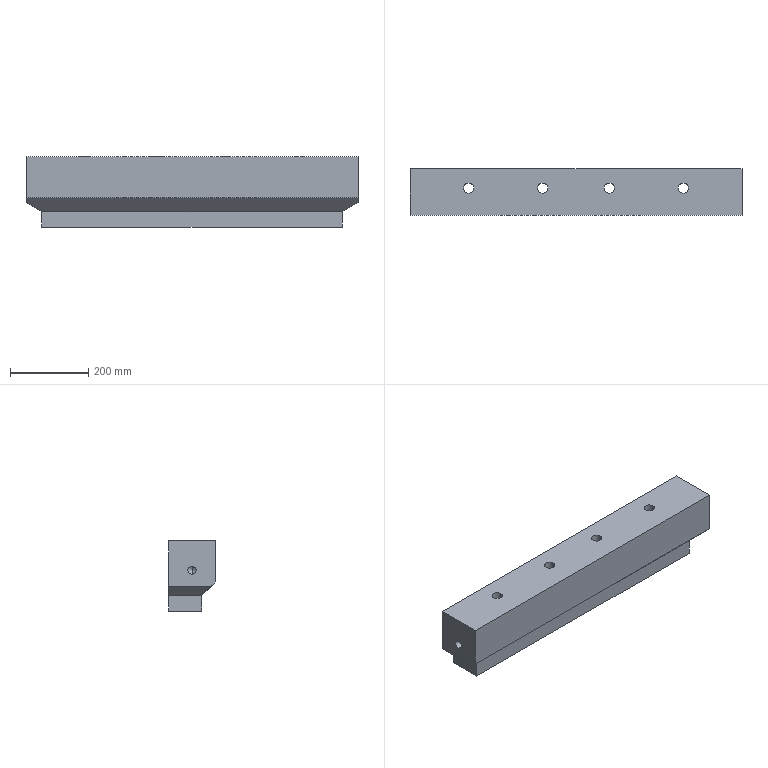Part | SolidWorks | features BaseBody 1 | 1 solid | 50 faces | box 850 x 120 x 180 mm | volume 15854243 mm3 | plane 26 | cylinder 16 | cone 8 | commonest cylinder face diameters 26 x8 17.5 x4 21 x4
STEP:
#1=CARTESIAN_POINT('',(-425.,-295.,-275.));
#2=VERTEX_POINT('',#1);
#3=CARTESIAN_POINT('',(-425.,-295.,-296.));
#4=VERTEX_POINT('',#3);
#5=CARTESIAN_POINT('',(-425.,-295.,-285.5));
#6=DIRECTION('',(1.,0.,0.));
#7=DIRECTION('',(0.,0.,-1.));
#8=AXIS2_PLACEMENT_3D('',#5,#6,#7);
#9=CIRCLE('',#8,10.5);
#10=EDGE_CURVE('',#2,#4,#9,.T.);
#11=ORIENTED_EDGE('',*,*,#10,.F.);
#12=CARTESIAN_POINT('',(-380.,-295.,-275.));
#13=VERTEX_POINT('',#12);
#14=CARTESIAN_POINT('',(-425.,-295.,-275.));
#15=DIRECTION('',(1.,0.,0.));
#16=VECTOR('',#15,1000.);
#17=LINE('',#14,#16);
#18=EDGE_CURVE('',#2,#13,#17,.T.);
#19=ORIENTED_EDGE('',*,*,#18,.T.);
#20=CARTESIAN_POINT('',(-380.,-295.,-296.));
#21=VERTEX_POINT('',#20);
#22=CARTESIAN_POINT('',(-380.,-295.,-285.5));
#23=DIRECTION('',(1.,0.,0.));
#24=DIRECTION('',(0.,0.,-1.));
#25=AXIS2_PLACEMENT_3D('',#22,#23,#24);
#26=CIRCLE('',#25,10.5);
#27=EDGE_CURVE('',#13,#21,#26,.T.);
#28=ORIENTED_EDGE('',*,*,#27,.T.);
#29=CARTESIAN_POINT('',(-425.,-295.,-296.));
#30=DIRECTION('',(1.,0.,0.));
#31=VECTOR('',#30,1000.);
#32=LINE('',#29,#31);
#33=EDGE_CURVE('',#4,#21,#32,.T.);
#34=ORIENTED_EDGE('',*,*,#33,.F.);
#35=EDGE_LOOP('',(#11,#19,#28,#34));
#36=FACE_OUTER_BOUND('',#35,.T.);
#37=CARTESIAN_POINT('',(-425.,-295.,-285.5));
#38=DIRECTION('',(1.,0.,0.));
#39=DIRECTION('',(0.,0.,-1.));
#40=AXIS2_PLACEMENT_3D('',#37,#38,#39);
#41=CYLINDRICAL_SURFACE('',#40,10.5);
#42=ADVANCED_FACE('',(#36),#41,.F.);
#43=CARTESIAN_POINT('',(-373.691,-295.,-285.5));
#44=VERTEX_POINT('',#43);
#45=CARTESIAN_POINT('',(-380.,-295.,-275.));
#46=DIRECTION('',(-0.515,0.,0.8572));
#47=VECTOR('',#46,1000.);
#48=LINE('',#45,#47);
#49=EDGE_CURVE('',#44,#13,#48,.T.);
#50=ORIENTED_EDGE('',*,*,#49,.F.);
#51=CARTESIAN_POINT('',(-380.,-295.,-296.));
#52=DIRECTION('',(-0.515,0.,-0.8572));
#53=VECTOR('',#52,1000.);
#54=LINE('',#51,#53);
#55=EDGE_CURVE('',#44,#21,#54,.T.);
#56=ORIENTED_EDGE('',*,*,#55,.T.);
#57=ORIENTED_EDGE('',*,*,#27,.F.);
#58=EDGE_LOOP('',(#50,#56,#57));
#59=FACE_OUTER_BOUND('',#58,.T.);
#60=CARTESIAN_POINT('',(-380.,-295.,-285.5));
#61=DIRECTION('',(-1.,0.,0.));
#62=DIRECTION('',(0.,0.,1.));
#63=AXIS2_PLACEMENT_3D('',#60,#61,#62);
#64=CONICAL_SURFACE('',#63,10.5,1.03);
#65=ADVANCED_FACE('',(#59),#64,.F.);
#66=CARTESIAN_POINT('',(425.,-295.,-296.));
#67=VERTEX_POINT('',#66);
#68=CARTESIAN_POINT('',(425.,-295.,-275.));
#69=VERTEX_POINT('',#68);
#70=CARTESIAN_POINT('',(425.,-295.,-285.5));
#71=DIRECTION('',(-1.,0.,0.));
#72=DIRECTION('',(0.,0.,1.));
#73=AXIS2_PLACEMENT_3D('',#70,#71,#72);
#74=CIRCLE('',#73,10.5);
#75=EDGE_CURVE('',#67,#69,#74,.T.);
#76=ORIENTED_EDGE('',*,*,#75,.F.);
#77=CARTESIAN_POINT('',(380.,-295.,-296.));
#78=VERTEX_POINT('',#77);
#79=CARTESIAN_POINT('',(425.,-295.,-296.));
#80=DIRECTION('',(-1.,0.,0.));
#81=VECTOR('',#80,1000.);
#82=LINE('',#79,#81);
#83=EDGE_CURVE('',#67,#78,#82,.T.);
#84=ORIENTED_EDGE('',*,*,#83,.T.);
#85=CARTESIAN_POINT('',(380.,-295.,-275.));
#86=VERTEX_POINT('',#85);
#87=CARTESIAN_POINT('',(380.,-295.,-285.5));
#88=DIRECTION('',(-1.,0.,0.));
#89=DIRECTION('',(0.,0.,1.));
#90=AXIS2_PLACEMENT_3D('',#87,#88,#89);
#91=CIRCLE('',#90,10.5);
#92=EDGE_CURVE('',#78,#86,#91,.T.);
#93=ORIENTED_EDGE('',*,*,#92,.T.);
#94=CARTESIAN_POINT('',(425.,-295.,-275.));
#95=DIRECTION('',(-1.,0.,0.));
#96=VECTOR('',#95,1000.);
#97=LINE('',#94,#96);
#98=EDGE_CURVE('',#69,#86,#97,.T.);
#99=ORIENTED_EDGE('',*,*,#98,.F.);
#100=EDGE_LOOP('',(#76,#84,#93,#99));
#101=FACE_OUTER_BOUND('',#100,.T.);
#102=CARTESIAN_POINT('',(425.,-295.,-285.5));
#103=DIRECTION('',(-1.,0.,0.));
#104=DIRECTION('',(0.,0.,1.));
#105=AXIS2_PLACEMENT_3D('',#102,#103,#104);
#106=CYLINDRICAL_SURFACE('',#105,10.5);
#107=ADVANCED_FACE('',(#101),#106,.F.);
#108=CARTESIAN_POINT('',(373.691,-295.,-285.5));
#109=VERTEX_POINT('',#108);
#110=CARTESIAN_POINT('',(380.,-295.,-296.));
#111=DIRECTION('',(0.515,0.,-0.8572));
#112=VECTOR('',#111,1000.);
#113=LINE('',#110,#112);
#114=EDGE_CURVE('',#109,#78,#113,.T.);
#115=ORIENTED_EDGE('',*,*,#114,.F.);
#116=CARTESIAN_POINT('',(380.,-295.,-275.));
#117=DIRECTION('',(0.515,0.,0.8572));
#118=VECTOR('',#117,1000.);
#119=LINE('',#116,#118);
#120=EDGE_CURVE('',#109,#86,#119,.T.);
#121=ORIENTED_EDGE('',*,*,#120,.T.);
#122=ORIENTED_EDGE('',*,*,#92,.F.);
#123=EDGE_LOOP('',(#115,#121,#122));
#124=FACE_OUTER_BOUND('',#123,.T.);
#125=CARTESIAN_POINT('',(380.,-295.,-285.5));
#126=DIRECTION('',(1.,0.,0.));
#127=DIRECTION('',(0.,0.,-1.));
#128=AXIS2_PLACEMENT_3D('',#125,#126,#127);
#129=CONICAL_SURFACE('',#128,10.5,1.03);
#130=ADVANCED_FACE('',(#124),#129,.F.);
#131=CARTESIAN_POINT('',(-353.75,-280.,-390.5));
#132=VERTEX_POINT('',#131);
#133=CARTESIAN_POINT('',(-336.25,-280.,-390.5));
#134=VERTEX_POINT('',#133);
#135=CARTESIAN_POINT('',(-345.,-280.,-390.5));
#136=DIRECTION('',(0.,0.,1.));
#137=DIRECTION('',(1.,0.,0.));
#138=AXIS2_PLACEMENT_3D('',#135,#136,#137);
#139=CIRCLE('',#138,8.75);
#140=EDGE_CURVE('',#132,#134,#139,.T.);
#141=ORIENTED_EDGE('',*,*,#140,.F.);
#142=CARTESIAN_POINT('',(-353.75,-280.,-345.5));
#143=VERTEX_POINT('',#142);
#144=CARTESIAN_POINT('',(-353.75,-280.,-390.5));
#145=DIRECTION('',(0.,0.,1.));
#146=VECTOR('',#145,1000.);
#147=LINE('',#144,#146);
#148=EDGE_CURVE('',#132,#143,#147,.T.);
#149=ORIENTED_EDGE('',*,*,#148,.T.);
#150=CARTESIAN_POINT('',(-336.25,-280.,-345.5));
#151=VERTEX_POINT('',#150);
#152=CARTESIAN_POINT('',(-345.,-280.,-345.5));
#153=DIRECTION('',(0.,0.,1.));
#154=DIRECTION('',(1.,0.,0.));
#155=AXIS2_PLACEMENT_3D('',#152,#153,#154);
#156=CIRCLE('',#155,8.75);
#157=EDGE_CURVE('',#143,#151,#156,.T.);
#158=ORIENTED_EDGE('',*,*,#157,.T.);
#159=CARTESIAN_POINT('',(-336.25,-280.,-390.5));
#160=DIRECTION('',(0.,0.,1.));
#161=VECTOR('',#160,1000.);
#162=LINE('',#159,#161);
#163=EDGE_CURVE('',#134,#151,#162,.T.);
#164=ORIENTED_EDGE('',*,*,#163,.F.);
#165=EDGE_LOOP('',(#141,#149,#158,#164));
#166=FACE_OUTER_BOUND('',#165,.T.);
#167=CARTESIAN_POINT('',(-345.,-280.,-390.5));
#168=DIRECTION('',(0.,0.,1.));
#169=DIRECTION('',(1.,0.,0.));
#170=AXIS2_PLACEMENT_3D('',#167,#168,#169);
#171=CYLINDRICAL_SURFACE('',#170,8.75);
#172=ADVANCED_FACE('',(#166),#171,.F.);
#173=CARTESIAN_POINT('',(-345.,-280.,-340.242));
#174=VERTEX_POINT('',#173);
#175=CARTESIAN_POINT('',(-353.75,-280.,-345.5));
#176=DIRECTION('',(-0.8572,0.,-0.515));
#177=VECTOR('',#176,1000.);
#178=LINE('',#175,#177);
#179=EDGE_CURVE('',#174,#143,#178,.T.);
#180=ORIENTED_EDGE('',*,*,#179,.F.);
#181=CARTESIAN_POINT('',(-336.25,-280.,-345.5));
#182=DIRECTION('',(0.8572,0.,-0.515));
#183=VECTOR('',#182,1000.);
#184=LINE('',#181,#183);
#185=EDGE_CURVE('',#174,#151,#184,.T.);
#186=ORIENTED_EDGE('',*,*,#185,.T.);
#187=ORIENTED_EDGE('',*,*,#157,.F.);
#188=EDGE_LOOP('',(#180,#186,#187));
#189=FACE_OUTER_BOUND('',#188,.T.);
#190=CARTESIAN_POINT('',(-345.,-280.,-345.5));
#191=DIRECTION('',(0.,0.,-1.));
#192=DIRECTION('',(-1.,0.,0.));
#193=AXIS2_PLACEMENT_3D('',#190,#191,#192);
#194=CONICAL_SURFACE('',#193,8.75,1.03);
#195=ADVANCED_FACE('',(#189),#194,.F.);
#196=CARTESIAN_POINT('',(336.25,-280.,-390.5));
#197=VERTEX_POINT('',#196);
#198=CARTESIAN_POINT('',(353.75,-280.,-390.5));
#199=VERTEX_POINT('',#198);
#200=CARTESIAN_POINT('',(345.,-280.,-390.5));
#201=DIRECTION('',(0.,0.,-1.));
#202=DIRECTION('',(-1.,0.,0.));
#203=AXIS2_PLACEMENT_3D('',#200,#201,#202);
#204=CIRCLE('',#203,8.75);
#205=EDGE_CURVE('',#197,#199,#204,.T.);
#206=ORIENTED_EDGE('',*,*,#205,.T.);
#207=CARTESIAN_POINT('',(353.75,-280.,-345.5));
#208=VERTEX_POINT('',#207);
#209=CARTESIAN_POINT('',(353.75,-280.,-390.5));
#210=DIRECTION('',(0.,0.,1.));
#211=VECTOR('',#210,1000.);
#212=LINE('',#209,#211);
#213=EDGE_CURVE('',#199,#208,#212,.T.);
#214=ORIENTED_EDGE('',*,*,#213,.T.);
#215=CARTESIAN_POINT('',(336.25,-280.,-345.5));
#216=VERTEX_POINT('',#215);
#217=CARTESIAN_POINT('',(345.,-280.,-345.5));
#218=DIRECTION('',(0.,0.,-1.));
#219=DIRECTION('',(-1.,0.,0.));
#220=AXIS2_PLACEMENT_3D('',#217,#218,#219);
#221=CIRCLE('',#220,8.75);
#222=EDGE_CURVE('',#216,#208,#221,.T.);
#223=ORIENTED_EDGE('',*,*,#222,.F.);
#224=CARTESIAN_POINT('',(336.25,-280.,-390.5));
#225=DIRECTION('',(0.,0.,1.));
#226=VECTOR('',#225,1000.);
#227=LINE('',#224,#226);
#228=EDGE_CURVE('',#197,#216,#227,.T.);
#229=ORIENTED_EDGE('',*,*,#228,.F.);
#230=EDGE_LOOP('',(#206,#214,#223,#229));
#231=FACE_OUTER_BOUND('',#230,.T.);
#232=CARTESIAN_POINT('',(345.,-280.,-390.5));
#233=DIRECTION('',(0.,0.,1.));
#234=DIRECTION('',(-1.,0.,0.));
#235=AXIS2_PLACEMENT_3D('',#232,#233,#234);
#236=CYLINDRICAL_SURFACE('',#235,8.75);
#237=ADVANCED_FACE('',(#231),#236,.F.);
#238=CARTESIAN_POINT('',(345.,-280.,-340.242));
#239=VERTEX_POINT('',#238);
#240=CARTESIAN_POINT('',(353.75,-280.,-345.5));
#241=DIRECTION('',(0.8572,0.,-0.515));
#242=VECTOR('',#241,1000.);
#243=LINE('',#240,#242);
#244=EDGE_CURVE('',#239,#208,#243,.T.);
#245=ORIENTED_EDGE('',*,*,#244,.F.);
#246=CARTESIAN_POINT('',(336.25,-280.,-345.5));
#247=DIRECTION('',(-0.8572,0.,-0.515));
#248=VECTOR('',#247,1000.);
#249=LINE('',#246,#248);
#250=EDGE_CURVE('',#239,#216,#249,.T.);
#251=ORIENTED_EDGE('',*,*,#250,.T.);
#252=ORIENTED_EDGE('',*,*,#222,.T.);
#253=EDGE_LOOP('',(#245,#251,#252));
#254=FACE_OUTER_BOUND('',#253,.T.);
#255=CARTESIAN_POINT('',(345.,-280.,-345.5));
#256=DIRECTION('',(0.,0.,-1.));
#257=DIRECTION('',(1.,0.,0.));
#258=AXIS2_PLACEMENT_3D('',#255,#256,#257);
#259=CONICAL_SURFACE('',#258,8.75,1.03);
#260=ADVANCED_FACE('',(#254),#259,.F.);
#261=CARTESIAN_POINT('',(-288.,-285.,-390.5));
#262=VERTEX_POINT('',#261);
#263=CARTESIAN_POINT('',(-262.,-285.,-390.5));
#264=VERTEX_POINT('',#263);
#265=CARTESIAN_POINT('',(-275.,-285.,-390.5));
#266=DIRECTION('',(0.,0.,1.));
#267=DIRECTION('',(1.,0.,0.));
#268=AXIS2_PLACEMENT_3D('',#265,#266,#267);
#269=CIRCLE('',#268,13.);
#270=EDGE_CURVE('',#262,#264,#269,.T.);
#271=ORIENTED_EDGE('',*,*,#270,.F.);
#272=CARTESIAN_POINT('',(-288.,-285.,-210.5));
#273=VERTEX_POINT('',#272);
#274=CARTESIAN_POINT('',(-288.,-285.,-395.5));
#275=DIRECTION('',(0.,0.,1.));
#276=VECTOR('',#275,1000.);
#277=LINE('',#274,#276);
#278=EDGE_CURVE('',#262,#273,#277,.T.);
#279=ORIENTED_EDGE('',*,*,#278,.T.);
#280=CARTESIAN_POINT('',(-262.,-285.,-210.5));
#281=VERTEX_POINT('',#280);
#282=CARTESIAN_POINT('',(-275.,-285.,-210.5));
#283=DIRECTION('',(0.,0.,1.));
#284=DIRECTION('',(1.,0.,0.));
#285=AXIS2_PLACEMENT_3D('',#282,#283,#284);
#286=CIRCLE('',#285,13.);
#287=EDGE_CURVE('',#273,#281,#286,.T.);
#288=ORIENTED_EDGE('',*,*,#287,.T.);
#289=CARTESIAN_POINT('',(-262.,-285.,-395.5));
#290=DIRECTION('',(0.,0.,1.));
#291=VECTOR('',#290,1000.);
#292=LINE('',#289,#291);
#293=EDGE_CURVE('',#264,#281,#292,.T.);
#294=ORIENTED_EDGE('',*,*,#293,.F.);
#295=EDGE_LOOP('',(#271,#279,#288,#294));
#296=FACE_OUTER_BOUND('',#295,.T.);
#297=CARTESIAN_POINT('',(-275.,-285.,-395.5));
#298=DIRECTION('',(0.,0.,1.));
#299=DIRECTION('',(1.,0.,0.));
#300=AXIS2_PLACEMENT_3D('',#297,#298,#299);
#301=CYLINDRICAL_SURFACE('',#300,13.);
#302=ADVANCED_FACE('',(#296),#301,.F.);
#303=CARTESIAN_POINT('',(262.,-285.,-390.5));
#304=VERTEX_POINT('',#303);
#305=CARTESIAN_POINT('',(288.,-285.,-390.5));
#306=VERTEX_POINT('',#305);
#307=CARTESIAN_POINT('',(275.,-285.,-390.5));
#308=DIRECTION('',(0.,0.,1.));
#309=DIRECTION('',(1.,0.,0.));
#310=AXIS2_PLACEMENT_3D('',#307,#308,#309);
#311=CIRCLE('',#310,13.);
#312=EDGE_CURVE('',#304,#306,#311,.T.);
#313=ORIENTED_EDGE('',*,*,#312,.F.);
#314=CARTESIAN_POINT('',(262.,-285.,-210.5));
#315=VERTEX_POINT('',#314);
#316=CARTESIAN_POINT('',(262.,-285.,-395.5));
#317=DIRECTION('',(0.,0.,1.));
#318=VECTOR('',#317,1000.);
#319=LINE('',#316,#318);
#320=EDGE_CURVE('',#304,#315,#319,.T.);
#321=ORIENTED_EDGE('',*,*,#320,.T.);
#322=CARTESIAN_POINT('',(288.,-285.,-210.5));
#323=VERTEX_POINT('',#322);
#324=CARTESIAN_POINT('',(275.,-285.,-210.5));
#325=DIRECTION('',(0.,0.,1.));
#326=DIRECTION('',(1.,0.,0.));
#327=AXIS2_PLACEMENT_3D('',#324,#325,#326);
#328=CIRCLE('',#327,13.);
#329=EDGE_CURVE('',#315,#323,#328,.T.);
#330=ORIENTED_EDGE('',*,*,#329,.T.);
#331=CARTESIAN_POINT('',(288.,-285.,-395.5));
#332=DIRECTION('',(0.,0.,1.));
#333=VECTOR('',#332,1000.);
#334=LINE('',#331,#333);
#335=EDGE_CURVE('',#306,#323,#334,.T.);
#336=ORIENTED_EDGE('',*,*,#335,.F.);
#337=EDGE_LOOP('',(#313,#321,#330,#336));
#338=FACE_OUTER_BOUND('',#337,.T.);
#339=CARTESIAN_POINT('',(275.,-285.,-395.5));
#340=DIRECTION('',(0.,0.,1.));
#341=DIRECTION('',(1.,0.,0.));
#342=AXIS2_PLACEMENT_3D('',#339,#340,#341);
#343=CYLINDRICAL_SURFACE('',#342,13.);
#344=ADVANCED_FACE('',(#338),#343,.F.);
#345=CARTESIAN_POINT('',(-98.,-285.,-390.5));
#346=VERTEX_POINT('',#345);
#347=CARTESIAN_POINT('',(-72.,-285.,-390.5));
#348=VERTEX_POINT('',#347);
#349=CARTESIAN_POINT('',(-85.,-285.,-390.5));
#350=DIRECTION('',(0.,0.,1.));
#351=DIRECTION('',(1.,0.,0.));
#352=AXIS2_PLACEMENT_3D('',#349,#350,#351);
#353=CIRCLE('',#352,13.);
#354=EDGE_CURVE('',#346,#348,#353,.T.);
#355=ORIENTED_EDGE('',*,*,#354,.F.);
#356=CARTESIAN_POINT('',(-98.,-285.,-210.5));
#357=VERTEX_POINT('',#356);
#358=CARTESIAN_POINT('',(-98.,-285.,-390.5));
#359=DIRECTION('',(0.,0.,1.));
#360=VECTOR('',#359,1000.);
#361=LINE('',#358,#360);
#362=EDGE_CURVE('',#346,#357,#361,.T.);
#363=ORIENTED_EDGE('',*,*,#362,.T.);
#364=CARTESIAN_POINT('',(-72.,-285.,-210.5));
#365=VERTEX_POINT('',#364);
#366=CARTESIAN_POINT('',(-85.,-285.,-210.5));
#367=DIRECTION('',(0.,0.,1.));
#368=DIRECTION('',(1.,0.,0.));
#369=AXIS2_PLACEMENT_3D('',#366,#367,#368);
#370=CIRCLE('',#369,13.);
#371=EDGE_CURVE('',#357,#365,#370,.T.);
#372=ORIENTED_EDGE('',*,*,#371,.T.);
#373=CARTESIAN_POINT('',(-72.,-285.,-390.5));
#374=DIRECTION('',(0.,0.,1.));
#375=VECTOR('',#374,1000.);
#376=LINE('',#373,#375);
#377=EDGE_CURVE('',#348,#365,#376,.T.);
#378=ORIENTED_EDGE('',*,*,#377,.F.);
#379=EDGE_LOOP('',(#355,#363,#372,#378));
#380=FACE_OUTER_BOUND('',#379,.T.);
#381=CARTESIAN_POINT('',(-85.,-285.,-390.5));
#382=DIRECTION('',(0.,0.,1.));
#383=DIRECTION('',(1.,0.,0.));
#384=AXIS2_PLACEMENT_3D('',#381,#382,#383);
#385=CYLINDRICAL_SURFACE('',#384,13.);
#386=ADVANCED_FACE('',(#380),#385,.F.);
#387=CARTESIAN_POINT('',(72.,-285.,-390.5));
#388=VERTEX_POINT('',#387);
#389=CARTESIAN_POINT('',(98.,-285.,-390.5));
#390=VERTEX_POINT('',#389);
#391=CARTESIAN_POINT('',(85.,-285.,-390.5));
#392=DIRECTION('',(0.,0.,1.));
#393=DIRECTION('',(1.,0.,0.));
#394=AXIS2_PLACEMENT_3D('',#391,#392,#393);
#395=CIRCLE('',#394,13.);
#396=EDGE_CURVE('',#388,#390,#395,.T.);
#397=ORIENTED_EDGE('',*,*,#396,.F.);
#398=CARTESIAN_POINT('',(72.,-285.,-210.5));
#399=VERTEX_POINT('',#398);
#400=CARTESIAN_POINT('',(72.,-285.,-390.5));
#401=DIRECTION('',(0.,0.,1.));
#402=VECTOR('',#401,1000.);
#403=LINE('',#400,#402);
#404=EDGE_CURVE('',#388,#399,#403,.T.);
#405=ORIENTED_EDGE('',*,*,#404,.T.);
#406=CARTESIAN_POINT('',(98.,-285.,-210.5));
#407=VERTEX_POINT('',#406);
#408=CARTESIAN_POINT('',(85.,-285.,-210.5));
#409=DIRECTION('',(0.,0.,1.));
#410=DIRECTION('',(1.,0.,0.));
#411=AXIS2_PLACEMENT_3D('',#408,#409,#410);
#412=CIRCLE('',#411,13.);
#413=EDGE_CURVE('',#399,#407,#412,.T.);
#414=ORIENTED_EDGE('',*,*,#413,.T.);
#415=CARTESIAN_POINT('',(98.,-285.,-390.5));
#416=DIRECTION('',(0.,0.,1.));
#417=VECTOR('',#416,1000.);
#418=LINE('',#415,#417);
#419=EDGE_CURVE('',#390,#407,#418,.T.);
#420=ORIENTED_EDGE('',*,*,#419,.F.);
#421=EDGE_LOOP('',(#397,#405,#414,#420));
#422=FACE_OUTER_BOUND('',#421,.T.);
#423=CARTESIAN_POINT('',(85.,-285.,-390.5));
#424=DIRECTION('',(0.,0.,1.));
#425=DIRECTION('',(1.,0.,0.));
#426=AXIS2_PLACEMENT_3D('',#423,#424,#425);
#427=CYLINDRICAL_SURFACE('',#426,13.);
#428=ADVANCED_FACE('',(#422),#427,.F.);
#429=CARTESIAN_POINT('',(-425.,-295.,-285.5));
#430=DIRECTION('',(1.,0.,0.));
#431=DIRECTION('',(0.,0.,-1.));
#432=AXIS2_PLACEMENT_3D('',#429,#430,#431);
#433=CIRCLE('',#432,10.5);
#434=EDGE_CURVE('',#4,#2,#433,.T.);
#435=ORIENTED_EDGE('',*,*,#434,.T.);
#436=ORIENTED_EDGE('',*,*,#10,.T.);
#437=EDGE_LOOP('',(#435,#436));
#438=FACE_BOUND('',#437,.T.);
#439=CARTESIAN_POINT('',(-425.,-235.,-327.406));
#440=VERTEX_POINT('',#439);
#441=CARTESIAN_POINT('',(-425.,-235.,-210.5));
#442=VERTEX_POINT('',#441);
#443=CARTESIAN_POINT('',(-425.,-235.,-390.5));
#444=DIRECTION('',(0.,0.,1.));
#445=VECTOR('',#444,1000.);
#446=LINE('',#443,#445);
#447=EDGE_CURVE('',#440,#442,#446,.T.);
#448=ORIENTED_EDGE('',*,*,#447,.F.);
#449=CARTESIAN_POINT('',(-425.,-343.094,-327.406));
#450=VERTEX_POINT('',#449);
#451=CARTESIAN_POINT('',(-425.,277.5,-327.406));
#452=DIRECTION('',(0.,-1.,0.));
#453=VECTOR('',#452,1000.);
#454=LINE('',#451,#453);
#455=EDGE_CURVE('',#440,#450,#454,.T.);
#456=ORIENTED_EDGE('',*,*,#455,.T.);
#457=CARTESIAN_POINT('',(-425.,-355.,-315.5));
#458=VERTEX_POINT('',#457);
#459=CARTESIAN_POINT('',(-425.,-320.,-350.5));
#460=DIRECTION('',(0.,-0.7071,0.7071));
#461=VECTOR('',#460,1000.);
#462=LINE('',#459,#461);
#463=EDGE_CURVE('',#450,#458,#462,.T.);
#464=ORIENTED_EDGE('',*,*,#463,.T.);
#465=CARTESIAN_POINT('',(-425.,-355.,-210.5));
#466=VERTEX_POINT('',#465);
#467=CARTESIAN_POINT('',(-425.,-355.,-390.5));
#468=DIRECTION('',(0.,0.,1.));
#469=VECTOR('',#468,1000.);
#470=LINE('',#467,#469);
#471=EDGE_CURVE('',#458,#466,#470,.T.);
#472=ORIENTED_EDGE('',*,*,#471,.T.);
#473=CARTESIAN_POINT('',(-425.,-235.,-210.5));
#474=DIRECTION('',(0.,-1.,0.));
#475=VECTOR('',#474,1000.);
#476=LINE('',#473,#475);
#477=EDGE_CURVE('',#442,#466,#476,.T.);
#478=ORIENTED_EDGE('',*,*,#477,.F.);
#479=EDGE_LOOP('',(#448,#456,#464,#472,#478));
#480=FACE_OUTER_BOUND('',#479,.T.);
#481=CARTESIAN_POINT('',(-425.,-235.,-390.5));
#482=DIRECTION('',(-1.,0.,0.));
#483=DIRECTION('',(0.,-1.,0.));
#484=AXIS2_PLACEMENT_3D('',#481,#482,#483);
#485=PLANE('',#484);
#486=ADVANCED_FACE('',(#438,#480),#485,.T.);
#487=CARTESIAN_POINT('',(375.662,-297.777,-390.5));
#488=VERTEX_POINT('',#487);
#489=CARTESIAN_POINT('',(375.662,-289.777,-390.5));
#490=VERTEX_POINT('',#489);
#491=CARTESIAN_POINT('',(375.662,-297.777,-390.5));
#492=DIRECTION('',(0.,1.,0.));
#493=VECTOR('',#492,1000.);
#494=LINE('',#491,#493);
#495=EDGE_CURVE('',#488,#490,#494,.T.);
#496=ORIENTED_EDGE('',*,*,#495,.F.);
#497=CARTESIAN_POINT('',(365.662,-297.777,-390.5));
#498=VERTEX_POINT('',#497);
#499=CARTESIAN_POINT('',(375.662,-297.777,-390.5));
#500=DIRECTION('',(-1.,0.,0.));
#501=VECTOR('',#500,1000.);
#502=LINE('',#499,#501);
#503=EDGE_CURVE('',#488,#498,#502,.T.);
#504=ORIENTED_EDGE('',*,*,#503,.T.);
#505=CARTESIAN_POINT('',(365.662,-307.777,-390.5));
#506=VERTEX_POINT('',#505);
#507=CARTESIAN_POINT('',(365.662,-307.777,-390.5));
#508=DIRECTION('',(0.,1.,0.));
#509=VECTOR('',#508,1000.);
#510=LINE('',#507,#509);
#511=EDGE_CURVE('',#506,#498,#510,.T.);
#512=ORIENTED_EDGE('',*,*,#511,.F.);
#513=CARTESIAN_POINT('',(357.662,-307.777,-390.5));
#514=VERTEX_POINT('',#513);
#515=CARTESIAN_POINT('',(365.662,-307.777,-390.5));
#516=DIRECTION('',(-1.,0.,0.));
#517=VECTOR('',#516,1000.);
#518=LINE('',#515,#517);
#519=EDGE_CURVE('',#506,#514,#518,.T.);
#520=ORIENTED_EDGE('',*,*,#519,.T.);
#521=CARTESIAN_POINT('',(357.662,-309.777,-390.5));
#522=VERTEX_POINT('',#521);
#523=CARTESIAN_POINT('',(357.662,-307.777,-390.5));
#524=DIRECTION('',(0.,-1.,0.));
#525=VECTOR('',#524,1000.);
#526=LINE('',#523,#525);
#527=EDGE_CURVE('',#514,#522,#526,.T.);
#528=ORIENTED_EDGE('',*,*,#527,.T.);
#529=CARTESIAN_POINT('',(377.662,-309.777,-390.5));
#530=VERTEX_POINT('',#529);
#531=CARTESIAN_POINT('',(377.662,-309.777,-390.5));
#532=DIRECTION('',(-1.,0.,0.));
#533=VECTOR('',#532,1000.);
#534=LINE('',#531,#533);
#535=EDGE_CURVE('',#530,#522,#534,.T.);
#536=ORIENTED_EDGE('',*,*,#535,.F.);
#537=CARTESIAN_POINT('',(377.662,-289.777,-390.5));
#538=VERTEX_POINT('',#537);
#539=CARTESIAN_POINT('',(377.662,-309.777,-390.5));
#540=DIRECTION('',(0.,1.,0.));
#541=VECTOR('',#540,1000.);
#542=LINE('',#539,#541);
#543=EDGE_CURVE('',#530,#538,#542,.T.);
#544=ORIENTED_EDGE('',*,*,#543,.T.);
#545=CARTESIAN_POINT('',(377.662,-289.777,-390.5));
#546=DIRECTION('',(-1.,0.,0.));
#547=VECTOR('',#546,1000.);
#548=LINE('',#545,#547);
#549=EDGE_CURVE('',#538,#490,#548,.T.);
#550=ORIENTED_EDGE('',*,*,#549,.T.);
#551=EDGE_LOOP('',(#496,#504,#512,#520,#528,#536,#544,#550));
#552=FACE_BOUND('',#551,.T.);
#553=CARTESIAN_POINT('',(-345.,-280.,-390.5));
#554=DIRECTION('',(0.,0.,1.));
#555=DIRECTION('',(1.,0.,0.));
#556=AXIS2_PLACEMENT_3D('',#553,#554,#555);
#557=CIRCLE('',#556,8.75);
#558=EDGE_CURVE('',#134,#132,#557,.T.);
#559=ORIENTED_EDGE('',*,*,#558,.T.);
#560=ORIENTED_EDGE('',*,*,#140,.T.);
#561=EDGE_LOOP('',(#559,#560));
#562=FACE_BOUND('',#561,.T.);
#563=CARTESIAN_POINT('',(-385.,-235.,-390.5));
#564=VERTEX_POINT('',#563);
#565=CARTESIAN_POINT('',(-385.,-320.,-390.5));
#566=VERTEX_POINT('',#565);
#567=CARTESIAN_POINT('',(-385.,-277.5,-390.5));
#568=DIRECTION('',(0.,-1.,0.));
#569=VECTOR('',#568,1000.);
#570=LINE('',#567,#569);
#571=EDGE_CURVE('',#564,#566,#570,.T.);
#572=ORIENTED_EDGE('',*,*,#571,.F.);
#573=CARTESIAN_POINT('',(385.,-235.,-390.5));
#574=VERTEX_POINT('',#573);
#575=CARTESIAN_POINT('',(425.,-235.,-390.5));
#576=DIRECTION('',(-1.,0.,0.));
#577=VECTOR('',#576,1000.);
#578=LINE('',#575,#577);
#579=EDGE_CURVE('',#574,#564,#578,.T.);
#580=ORIENTED_EDGE('',*,*,#579,.F.);
#581=CARTESIAN_POINT('',(385.,-320.,-390.5));
#582=VERTEX_POINT('',#581);
#583=CARTESIAN_POINT('',(385.,-355.,-390.5));
#584=DIRECTION('',(0.,-1.,0.));
#585=VECTOR('',#584,1000.);
#586=LINE('',#583,#585);
#587=EDGE_CURVE('',#574,#582,#586,.T.);
#588=ORIENTED_EDGE('',*,*,#587,.T.);
#589=CARTESIAN_POINT('',(510.,-320.,-390.5));
#590=DIRECTION('',(-1.,0.,0.));
#591=VECTOR('',#590,1000.);
#592=LINE('',#589,#591);
#593=EDGE_CURVE('',#582,#566,#592,.T.);
#594=ORIENTED_EDGE('',*,*,#593,.T.);
#595=EDGE_LOOP('',(#572,#580,#588,#594));
#596=FACE_OUTER_BOUND('',#595,.T.);
#597=CARTESIAN_POINT('',(-85.,-285.,-390.5));
#598=DIRECTION('',(0.,0.,1.));
#599=DIRECTION('',(1.,0.,0.));
#600=AXIS2_PLACEMENT_3D('',#597,#598,#599);
#601=CIRCLE('',#600,13.);
#602=EDGE_CURVE('',#348,#346,#601,.T.);
#603=ORIENTED_EDGE('',*,*,#602,.T.);
#604=ORIENTED_EDGE('',*,*,#354,.T.);
#605=EDGE_LOOP('',(#603,#604));
#606=FACE_BOUND('',#605,.T.);
#607=CARTESIAN_POINT('',(85.,-285.,-390.5));
#608=DIRECTION('',(0.,0.,1.));
#609=DIRECTION('',(1.,0.,0.));
#610=AXIS2_PLACEMENT_3D('',#607,#608,#609);
#611=CIRCLE('',#610,13.);
#612=EDGE_CURVE('',#390,#388,#611,.T.);
#613=ORIENTED_EDGE('',*,*,#612,.T.);
#614=ORIENTED_EDGE('',*,*,#396,.T.);
#615=EDGE_LOOP('',(#613,#614));
#616=FACE_BOUND('',#615,.T.);
#617=CARTESIAN_POINT('',(275.,-285.,-390.5));
#618=DIRECTION('',(0.,0.,1.));
#619=DIRECTION('',(1.,0.,0.));
#620=AXIS2_PLACEMENT_3D('',#617,#618,#619);
#621=CIRCLE('',#620,13.);
#622=EDGE_CURVE('',#306,#304,#621,.T.);
#623=ORIENTED_EDGE('',*,*,#622,.T.);
#624=ORIENTED_EDGE('',*,*,#312,.T.);
#625=EDGE_LOOP('',(#623,#624));
#626=FACE_BOUND('',#625,.T.);
#627=CARTESIAN_POINT('',(-275.,-285.,-390.5));
#628=DIRECTION('',(0.,0.,1.));
#629=DIRECTION('',(1.,0.,0.));
#630=AXIS2_PLACEMENT_3D('',#627,#628,#629);
#631=CIRCLE('',#630,13.);
#632=EDGE_CURVE('',#264,#262,#631,.T.);
#633=ORIENTED_EDGE('',*,*,#632,.T.);
#634=ORIENTED_EDGE('',*,*,#270,.T.);
#635=EDGE_LOOP('',(#633,#634));
#636=FACE_BOUND('',#635,.T.);
#637=ORIENTED_EDGE('',*,*,#205,.F.);
#638=CARTESIAN_POINT('',(345.,-280.,-390.5));
#639=DIRECTION('',(0.,0.,-1.));
#640=DIRECTION('',(-1.,0.,0.));
#641=AXIS2_PLACEMENT_3D('',#638,#639,#640);
#642=CIRCLE('',#641,8.75);
#643=EDGE_CURVE('',#199,#197,#642,.T.);
#644=ORIENTED_EDGE('',*,*,#643,.F.);
#645=EDGE_LOOP('',(#637,#644));
#646=FACE_BOUND('',#645,.T.);
#647=CARTESIAN_POINT('',(-425.,-355.,-390.5));
#648=DIRECTION('',(0.,0.,1.));
#649=DIRECTION('',(1.,0.,0.));
#650=AXIS2_PLACEMENT_3D('',#647,#648,#649);
#651=PLANE('',#650);
#652=ADVANCED_FACE('',(#552,#562,#596,#606,#616,#626,#636,#646),#651,.F.);
#653=ORIENTED_EDGE('',*,*,#579,.T.);
#654=CARTESIAN_POINT('',(-385.,-235.,-350.5));
#655=VERTEX_POINT('',#654);
#656=CARTESIAN_POINT('',(-385.,-235.,-390.5));
#657=DIRECTION('',(0.,0.,1.));
#658=VECTOR('',#657,1000.);
#659=LINE('',#656,#658);
#660=EDGE_CURVE('',#564,#655,#659,.T.);
#661=ORIENTED_EDGE('',*,*,#660,.T.);
#662=CARTESIAN_POINT('',(-385.,-235.,-350.5));
#663=DIRECTION('',(-0.866,0.,0.5));
#664=VECTOR('',#663,1000.);
#665=LINE('',#662,#664);
#666=EDGE_CURVE('',#655,#440,#665,.T.);
#667=ORIENTED_EDGE('',*,*,#666,.T.);
#668=ORIENTED_EDGE('',*,*,#447,.T.);
#669=CARTESIAN_POINT('',(425.,-235.,-210.5));
#670=VERTEX_POINT('',#669);
#671=CARTESIAN_POINT('',(425.,-235.,-210.5));
#672=DIRECTION('',(-1.,0.,0.));
#673=VECTOR('',#672,1000.);
#674=LINE('',#671,#673);
#675=EDGE_CURVE('',#670,#442,#674,.T.);
#676=ORIENTED_EDGE('',*,*,#675,.F.);
#677=CARTESIAN_POINT('',(425.,-235.,-327.406));
#678=VERTEX_POINT('',#677);
#679=CARTESIAN_POINT('',(425.,-235.,-390.5));
#680=DIRECTION('',(0.,0.,1.));
#681=VECTOR('',#680,1000.);
#682=LINE('',#679,#681);
#683=EDGE_CURVE('',#678,#670,#682,.T.);
#684=ORIENTED_EDGE('',*,*,#683,.F.);
#685=CARTESIAN_POINT('',(385.,-235.,-350.5));
#686=VERTEX_POINT('',#685);
#687=CARTESIAN_POINT('',(397.679,-235.,-343.179));
#688=DIRECTION('',(0.866,0.,0.5));
#689=VECTOR('',#688,1000.);
#690=LINE('',#687,#689);
#691=EDGE_CURVE('',#686,#678,#690,.T.);
#692=ORIENTED_EDGE('',*,*,#691,.F.);
#693=CARTESIAN_POINT('',(385.,-235.,-390.5));
#694=DIRECTION('',(0.,0.,1.));
#695=VECTOR('',#694,1000.);
#696=LINE('',#693,#695);
#697=EDGE_CURVE('',#574,#686,#696,.T.);
#698=ORIENTED_EDGE('',*,*,#697,.F.);
#699=EDGE_LOOP('',(#653,#661,#667,#668,#676,#684,#692,#698));
#700=FACE_OUTER_BOUND('',#699,.T.);
#701=CARTESIAN_POINT('',(425.,-235.,-390.5));
#702=DIRECTION('',(0.,1.,0.));
#703=DIRECTION('',(0.,0.,1.));
#704=AXIS2_PLACEMENT_3D('',#701,#702,#703);
#705=PLANE('',#704);
#706=ADVANCED_FACE('',(#700),#705,.T.);
#707=CARTESIAN_POINT('',(425.,-355.,-315.5));
#708=VERTEX_POINT('',#707);
#709=CARTESIAN_POINT('',(510.,-355.,-315.5));
#710=DIRECTION('',(-1.,0.,0.));
#711=VECTOR('',#710,1000.);
#712=LINE('',#709,#711);
#713=EDGE_CURVE('',#708,#458,#712,.T.);
#714=ORIENTED_EDGE('',*,*,#713,.F.);
#715=CARTESIAN_POINT('',(425.,-355.,-210.5));
#716=VERTEX_POINT('',#715);
#717=CARTESIAN_POINT('',(425.,-355.,-390.5));
#718=DIRECTION('',(0.,0.,1.));
#719=VECTOR('',#718,1000.);
#720=LINE('',#717,#719);
#721=EDGE_CURVE('',#708,#716,#720,.T.);
#722=ORIENTED_EDGE('',*,*,#721,.T.);
#723=CARTESIAN_POINT('',(-425.,-355.,-210.5));
#724=DIRECTION('',(1.,0.,0.));
#725=VECTOR('',#724,1000.);
#726=LINE('',#723,#725);
#727=EDGE_CURVE('',#466,#716,#726,.T.);
#728=ORIENTED_EDGE('',*,*,#727,.F.);
#729=ORIENTED_EDGE('',*,*,#471,.F.);
#730=EDGE_LOOP('',(#714,#722,#728,#729));
#731=FACE_OUTER_BOUND('',#730,.T.);
#732=CARTESIAN_POINT('',(-425.,-355.,-390.5));
#733=DIRECTION('',(0.,-1.,0.));
#734=DIRECTION('',(0.,0.,-1.));
#735=AXIS2_PLACEMENT_3D('',#732,#733,#734);
#736=PLANE('',#735);
#737=ADVANCED_FACE('',(#731),#736,.T.);
#738=CARTESIAN_POINT('',(425.,-295.,-285.5));
#739=DIRECTION('',(-1.,0.,0.));
#740=DIRECTION('',(0.,0.,1.));
#741=AXIS2_PLACEMENT_3D('',#738,#739,#740);
#742=CIRCLE('',#741,10.5);
#743=EDGE_CURVE('',#69,#67,#742,.T.);
#744=ORIENTED_EDGE('',*,*,#743,.T.);
#745=ORIENTED_EDGE('',*,*,#75,.T.);
#746=EDGE_LOOP('',(#744,#745));
#747=FACE_BOUND('',#746,.T.);
#748=CARTESIAN_POINT('',(425.,-343.094,-327.406));
#749=VERTEX_POINT('',#748);
#750=CARTESIAN_POINT('',(425.,-355.,-327.406));
#751=DIRECTION('',(0.,-1.,0.));
#752=VECTOR('',#751,1000.);
#753=LINE('',#750,#752);
#754=EDGE_CURVE('',#678,#749,#753,.T.);
#755=ORIENTED_EDGE('',*,*,#754,.F.);
#756=ORIENTED_EDGE('',*,*,#683,.T.);
#757=CARTESIAN_POINT('',(425.,-355.,-210.5));
#758=DIRECTION('',(0.,1.,0.));
#759=VECTOR('',#758,1000.);
#760=LINE('',#757,#759);
#761=EDGE_CURVE('',#716,#670,#760,.T.);
#762=ORIENTED_EDGE('',*,*,#761,.F.);
#763=ORIENTED_EDGE('',*,*,#721,.F.);
#764=CARTESIAN_POINT('',(425.,-320.,-350.5));
#765=DIRECTION('',(0.,-0.7071,0.7071));
#766=VECTOR('',#765,1000.);
#767=LINE('',#764,#766);
#768=EDGE_CURVE('',#749,#708,#767,.T.);
#769=ORIENTED_EDGE('',*,*,#768,.F.);
#770=EDGE_LOOP('',(#755,#756,#762,#763,#769));
#771=FACE_OUTER_BOUND('',#770,.T.);
#772=CARTESIAN_POINT('',(425.,-355.,-390.5));
#773=DIRECTION('',(1.,0.,0.));
#774=DIRECTION('',(0.,0.,-1.));
#775=AXIS2_PLACEMENT_3D('',#772,#773,#774);
#776=PLANE('',#775);
#777=ADVANCED_FACE('',(#747,#771),#776,.T.);
#778=CARTESIAN_POINT('',(-275.,-285.,-210.5));
#779=DIRECTION('',(0.,0.,1.));
#780=DIRECTION('',(1.,0.,0.));
#781=AXIS2_PLACEMENT_3D('',#778,#779,#780);
#782=CIRCLE('',#781,13.);
#783=EDGE_CURVE('',#281,#273,#782,.T.);
#784=ORIENTED_EDGE('',*,*,#783,.F.);
#785=ORIENTED_EDGE('',*,*,#287,.F.);
#786=EDGE_LOOP('',(#784,#785));
#787=FACE_BOUND('',#786,.T.);
#788=CARTESIAN_POINT('',(275.,-285.,-210.5));
#789=DIRECTION('',(0.,0.,1.));
#790=DIRECTION('',(1.,0.,0.));
#791=AXIS2_PLACEMENT_3D('',#788,#789,#790);
#792=CIRCLE('',#791,13.);
#793=EDGE_CURVE('',#323,#315,#792,.T.);
#794=ORIENTED_EDGE('',*,*,#793,.F.);
#795=ORIENTED_EDGE('',*,*,#329,.F.);
#796=EDGE_LOOP('',(#794,#795));
#797=FACE_BOUND('',#796,.T.);
#798=CARTESIAN_POINT('',(-85.,-285.,-210.5));
#799=DIRECTION('',(0.,0.,1.));
#800=DIRECTION('',(1.,0.,0.));
#801=AXIS2_PLACEMENT_3D('',#798,#799,#800);
#802=CIRCLE('',#801,13.);
#803=EDGE_CURVE('',#365,#357,#802,.T.);
#804=ORIENTED_EDGE('',*,*,#803,.F.);
#805=ORIENTED_EDGE('',*,*,#371,.F.);
#806=EDGE_LOOP('',(#804,#805));
#807=FACE_BOUND('',#806,.T.);
#808=CARTESIAN_POINT('',(85.,-285.,-210.5));
#809=DIRECTION('',(0.,0.,1.));
#810=DIRECTION('',(1.,0.,0.));
#811=AXIS2_PLACEMENT_3D('',#808,#809,#810);
#812=CIRCLE('',#811,13.);
#813=EDGE_CURVE('',#407,#399,#812,.T.);
#814=ORIENTED_EDGE('',*,*,#813,.F.);
#815=ORIENTED_EDGE('',*,*,#413,.F.);
#816=EDGE_LOOP('',(#814,#815));
#817=FACE_BOUND('',#816,.T.);
#818=ORIENTED_EDGE('',*,*,#477,.T.);
#819=ORIENTED_EDGE('',*,*,#727,.T.);
#820=ORIENTED_EDGE('',*,*,#761,.T.);
#821=ORIENTED_EDGE('',*,*,#675,.T.);
#822=EDGE_LOOP('',(#818,#819,#820,#821));
#823=FACE_OUTER_BOUND('',#822,.T.);
#824=CARTESIAN_POINT('',(-425.,-355.,-210.5));
#825=DIRECTION('',(0.,0.,1.));
#826=DIRECTION('',(1.,0.,0.));
#827=AXIS2_PLACEMENT_3D('',#824,#825,#826);
#828=PLANE('',#827);
#829=ADVANCED_FACE('',(#787,#797,#807,#817,#823),#828,.T.);
#830=ORIENTED_EDGE('',*,*,#404,.F.);
#831=ORIENTED_EDGE('',*,*,#612,.F.);
#832=ORIENTED_EDGE('',*,*,#419,.T.);
#833=ORIENTED_EDGE('',*,*,#813,.T.);
#834=EDGE_LOOP('',(#830,#831,#832,#833));
#835=FACE_OUTER_BOUND('',#834,.T.);
#836=CARTESIAN_POINT('',(85.,-285.,-390.5));
#837=DIRECTION('',(0.,0.,1.));
#838=DIRECTION('',(1.,0.,0.));
#839=AXIS2_PLACEMENT_3D('',#836,#837,#838);
#840=CYLINDRICAL_SURFACE('',#839,13.);
#841=ADVANCED_FACE('',(#835),#840,.F.);
#842=ORIENTED_EDGE('',*,*,#362,.F.);
#843=ORIENTED_EDGE('',*,*,#602,.F.);
#844=ORIENTED_EDGE('',*,*,#377,.T.);
#845=ORIENTED_EDGE('',*,*,#803,.T.);
#846=EDGE_LOOP('',(#842,#843,#844,#845));
#847=FACE_OUTER_BOUND('',#846,.T.);
#848=CARTESIAN_POINT('',(-85.,-285.,-390.5));
#849=DIRECTION('',(0.,0.,1.));
#850=DIRECTION('',(1.,0.,0.));
#851=AXIS2_PLACEMENT_3D('',#848,#849,#850);
#852=CYLINDRICAL_SURFACE('',#851,13.);
#853=ADVANCED_FACE('',(#847),#852,.F.);
#854=ORIENTED_EDGE('',*,*,#768,.T.);
#855=ORIENTED_EDGE('',*,*,#713,.T.);
#856=ORIENTED_EDGE('',*,*,#463,.F.);
#857=CARTESIAN_POINT('',(-385.,-320.,-350.5));
#858=VERTEX_POINT('',#857);
#859=CARTESIAN_POINT('',(-178.02,-200.5,-470.));
#860=DIRECTION('',(0.7746,0.4472,-0.4472));
#861=VECTOR('',#860,1000.);
#862=LINE('',#859,#861);
#863=EDGE_CURVE('',#450,#858,#862,.T.);
#864=ORIENTED_EDGE('',*,*,#863,.T.);
#865=CARTESIAN_POINT('',(385.,-320.,-350.5));
#866=VERTEX_POINT('',#865);
#867=CARTESIAN_POINT('',(510.,-320.,-350.5));
#868=DIRECTION('',(-1.,0.,0.));
#869=VECTOR('',#868,1000.);
#870=LINE('',#867,#869);
#871=EDGE_CURVE('',#866,#858,#870,.T.);
#872=ORIENTED_EDGE('',*,*,#871,.F.);
#873=CARTESIAN_POINT('',(460.,-363.301,-307.199));
#874=DIRECTION('',(-0.7746,0.4472,-0.4472));
#875=VECTOR('',#874,1000.);
#876=LINE('',#873,#875);
#877=EDGE_CURVE('',#749,#866,#876,.T.);
#878=ORIENTED_EDGE('',*,*,#877,.F.);
#879=EDGE_LOOP('',(#854,#855,#856,#864,#872,#878));
#880=FACE_OUTER_BOUND('',#879,.T.);
#881=CARTESIAN_POINT('',(510.,-320.,-350.5));
#882=DIRECTION('',(0.,-0.7071,-0.7071));
#883=DIRECTION('',(0.,0.7071,-0.7071));
#884=AXIS2_PLACEMENT_3D('',#881,#882,#883);
#885=PLANE('',#884);
#886=ADVANCED_FACE('',(#880),#885,.T.);
#887=CARTESIAN_POINT('',(-385.,-320.,-390.5));
#888=DIRECTION('',(0.,0.,1.));
#889=VECTOR('',#888,1000.);
#890=LINE('',#887,#889);
#891=EDGE_CURVE('',#566,#858,#890,.T.);
#892=ORIENTED_EDGE('',*,*,#891,.F.);
#893=ORIENTED_EDGE('',*,*,#593,.F.);
#894=CARTESIAN_POINT('',(385.,-320.,-390.5));
#895=DIRECTION('',(0.,0.,-1.));
#896=VECTOR('',#895,1000.);
#897=LINE('',#894,#896);
#898=EDGE_CURVE('',#866,#582,#897,.T.);
#899=ORIENTED_EDGE('',*,*,#898,.F.);
#900=ORIENTED_EDGE('',*,*,#871,.T.);
#901=EDGE_LOOP('',(#892,#893,#899,#900));
#902=FACE_OUTER_BOUND('',#901,.T.);
#903=CARTESIAN_POINT('',(510.,-320.,-390.5));
#904=DIRECTION('',(0.,-1.,0.));
#905=DIRECTION('',(0.,0.,-1.));
#906=AXIS2_PLACEMENT_3D('',#903,#904,#905);
#907=PLANE('',#906);
#908=ADVANCED_FACE('',(#902),#907,.T.);
#909=ORIENTED_EDGE('',*,*,#691,.T.);
#910=ORIENTED_EDGE('',*,*,#754,.T.);
#911=ORIENTED_EDGE('',*,*,#877,.T.);
#912=CARTESIAN_POINT('',(385.,-292.5,-350.5));
#913=DIRECTION('',(0.,1.,0.));
#914=VECTOR('',#913,1000.);
#915=LINE('',#912,#914);
#916=EDGE_CURVE('',#866,#686,#915,.T.);
#917=ORIENTED_EDGE('',*,*,#916,.T.);
#918=EDGE_LOOP('',(#909,#910,#911,#917));
#919=FACE_OUTER_BOUND('',#918,.T.);
#920=CARTESIAN_POINT('',(385.,-277.5,-350.5));
#921=DIRECTION('',(0.5,0.,-0.866));
#922=DIRECTION('',(-0.866,0.,-0.5));
#923=AXIS2_PLACEMENT_3D('',#920,#921,#922);
#924=PLANE('',#923);
#925=ADVANCED_FACE('',(#919),#924,.T.);
#926=ORIENTED_EDGE('',*,*,#697,.T.);
#927=ORIENTED_EDGE('',*,*,#916,.F.);
#928=ORIENTED_EDGE('',*,*,#898,.T.);
#929=ORIENTED_EDGE('',*,*,#587,.F.);
#930=EDGE_LOOP('',(#926,#927,#928,#929));
#931=FACE_OUTER_BOUND('',#930,.T.);
#932=CARTESIAN_POINT('',(385.,-292.5,-410.5));
#933=DIRECTION('',(-1.,0.,0.));
#934=DIRECTION('',(0.,0.,1.));
#935=AXIS2_PLACEMENT_3D('',#932,#933,#934);
#936=PLANE('',#935);
#937=ADVANCED_FACE('',(#931),#936,.F.);
#938=ORIENTED_EDGE('',*,*,#863,.F.);
#939=ORIENTED_EDGE('',*,*,#455,.F.);
#940=ORIENTED_EDGE('',*,*,#666,.F.);
#941=CARTESIAN_POINT('',(-385.,-277.5,-350.5));
#942=DIRECTION('',(0.,1.,0.));
#943=VECTOR('',#942,1000.);
#944=LINE('',#941,#943);
#945=EDGE_CURVE('',#858,#655,#944,.T.);
#946=ORIENTED_EDGE('',*,*,#945,.F.);
#947=EDGE_LOOP('',(#938,#939,#940,#946));
#948=FACE_OUTER_BOUND('',#947,.T.);
#949=CARTESIAN_POINT('',(-385.,277.5,-350.5));
#950=DIRECTION('',(-0.5,0.,-0.866));
#951=DIRECTION('',(-0.866,0.,0.5));
#952=AXIS2_PLACEMENT_3D('',#949,#950,#951);
#953=PLANE('',#952);
#954=ADVANCED_FACE('',(#948),#953,.T.);
#955=ORIENTED_EDGE('',*,*,#891,.T.);
#956=ORIENTED_EDGE('',*,*,#945,.T.);
#957=ORIENTED_EDGE('',*,*,#660,.F.);
#958=ORIENTED_EDGE('',*,*,#571,.T.);
#959=EDGE_LOOP('',(#955,#956,#957,#958));
#960=FACE_OUTER_BOUND('',#959,.T.);
#961=CARTESIAN_POINT('',(-385.,-277.5,-390.5));
#962=DIRECTION('',(1.,0.,0.));
#963=DIRECTION('',(0.,0.,1.));
#964=AXIS2_PLACEMENT_3D('',#961,#962,#963);
#965=PLANE('',#964);
#966=ADVANCED_FACE('',(#960),#965,.F.);
#967=ORIENTED_EDGE('',*,*,#320,.F.);
#968=ORIENTED_EDGE('',*,*,#622,.F.);
#969=ORIENTED_EDGE('',*,*,#335,.T.);
#970=ORIENTED_EDGE('',*,*,#793,.T.);
#971=EDGE_LOOP('',(#967,#968,#969,#970));
#972=FACE_OUTER_BOUND('',#971,.T.);
#973=CARTESIAN_POINT('',(275.,-285.,-395.5));
#974=DIRECTION('',(0.,0.,1.));
#975=DIRECTION('',(1.,0.,0.));
#976=AXIS2_PLACEMENT_3D('',#973,#974,#975);
#977=CYLINDRICAL_SURFACE('',#976,13.);
#978=ADVANCED_FACE('',(#972),#977,.F.);
#979=ORIENTED_EDGE('',*,*,#278,.F.);
#980=ORIENTED_EDGE('',*,*,#632,.F.);
#981=ORIENTED_EDGE('',*,*,#293,.T.);
#982=ORIENTED_EDGE('',*,*,#783,.T.);
#983=EDGE_LOOP('',(#979,#980,#981,#982));
#984=FACE_OUTER_BOUND('',#983,.T.);
#985=CARTESIAN_POINT('',(-275.,-285.,-395.5));
#986=DIRECTION('',(0.,0.,1.));
#987=DIRECTION('',(1.,0.,0.));
#988=AXIS2_PLACEMENT_3D('',#985,#986,#987);
#989=CYLINDRICAL_SURFACE('',#988,13.);
#990=ADVANCED_FACE('',(#984),#989,.F.);
#991=ORIENTED_EDGE('',*,*,#250,.F.);
#992=ORIENTED_EDGE('',*,*,#244,.T.);
#993=CARTESIAN_POINT('',(345.,-280.,-345.5));
#994=DIRECTION('',(0.,0.,-1.));
#995=DIRECTION('',(-1.,0.,0.));
#996=AXIS2_PLACEMENT_3D('',#993,#994,#995);
#997=CIRCLE('',#996,8.75);
#998=EDGE_CURVE('',#208,#216,#997,.T.);
#999=ORIENTED_EDGE('',*,*,#998,.T.);
#1000=EDGE_LOOP('',(#991,#992,#999));
#1001=FACE_OUTER_BOUND('',#1000,.T.);
#1002=CARTESIAN_POINT('',(345.,-280.,-345.5));
#1003=DIRECTION('',(0.,0.,-1.));
#1004=DIRECTION('',(1.,0.,0.));
#1005=AXIS2_PLACEMENT_3D('',#1002,#1003,#1004);
#1006=CONICAL_SURFACE('',#1005,8.75,1.03);
#1007=ADVANCED_FACE('',(#1001),#1006,.F.);
#1008=ORIENTED_EDGE('',*,*,#213,.F.);
#1009=ORIENTED_EDGE('',*,*,#643,.T.);
#1010=ORIENTED_EDGE('',*,*,#228,.T.);
#1011=ORIENTED_EDGE('',*,*,#998,.F.);
#1012=EDGE_LOOP('',(#1008,#1009,#1010,#1011));
#1013=FACE_OUTER_BOUND('',#1012,.T.);
#1014=CARTESIAN_POINT('',(345.,-280.,-390.5));
#1015=DIRECTION('',(0.,0.,1.));
#1016=DIRECTION('',(-1.,0.,0.));
#1017=AXIS2_PLACEMENT_3D('',#1014,#1015,#1016);
#1018=CYLINDRICAL_SURFACE('',#1017,8.75);
#1019=ADVANCED_FACE('',(#1013),#1018,.F.);
#1020=ORIENTED_EDGE('',*,*,#185,.F.);
#1021=ORIENTED_EDGE('',*,*,#179,.T.);
#1022=CARTESIAN_POINT('',(-345.,-280.,-345.5));
#1023=DIRECTION('',(0.,0.,1.));
#1024=DIRECTION('',(1.,0.,0.));
#1025=AXIS2_PLACEMENT_3D('',#1022,#1023,#1024);
#1026=CIRCLE('',#1025,8.75);
#1027=EDGE_CURVE('',#151,#143,#1026,.T.);
#1028=ORIENTED_EDGE('',*,*,#1027,.F.);
#1029=EDGE_LOOP('',(#1020,#1021,#1028));
#1030=FACE_OUTER_BOUND('',#1029,.T.);
#1031=CARTESIAN_POINT('',(-345.,-280.,-345.5));
#1032=DIRECTION('',(0.,0.,-1.));
#1033=DIRECTION('',(-1.,0.,0.));
#1034=AXIS2_PLACEMENT_3D('',#1031,#1032,#1033);
#1035=CONICAL_SURFACE('',#1034,8.75,1.03);
#1036=ADVANCED_FACE('',(#1030),#1035,.F.);
#1037=ORIENTED_EDGE('',*,*,#148,.F.);
#1038=ORIENTED_EDGE('',*,*,#558,.F.);
#1039=ORIENTED_EDGE('',*,*,#163,.T.);
#1040=ORIENTED_EDGE('',*,*,#1027,.T.);
#1041=EDGE_LOOP('',(#1037,#1038,#1039,#1040));
#1042=FACE_OUTER_BOUND('',#1041,.T.);
#1043=CARTESIAN_POINT('',(-345.,-280.,-390.5));
#1044=DIRECTION('',(0.,0.,1.));
#1045=DIRECTION('',(1.,0.,0.));
#1046=AXIS2_PLACEMENT_3D('',#1043,#1044,#1045);
#1047=CYLINDRICAL_SURFACE('',#1046,8.75);
#1048=ADVANCED_FACE('',(#1042),#1047,.F.);
#1049=ORIENTED_EDGE('',*,*,#120,.F.);
#1050=ORIENTED_EDGE('',*,*,#114,.T.);
#1051=CARTESIAN_POINT('',(380.,-295.,-285.5));
#1052=DIRECTION('',(-1.,0.,0.));
#1053=DIRECTION('',(0.,0.,1.));
#1054=AXIS2_PLACEMENT_3D('',#1051,#1052,#1053);
#1055=CIRCLE('',#1054,10.5);
#1056=EDGE_CURVE('',#86,#78,#1055,.T.);
#1057=ORIENTED_EDGE('',*,*,#1056,.F.);
#1058=EDGE_LOOP('',(#1049,#1050,#1057));
#1059=FACE_OUTER_BOUND('',#1058,.T.);
#1060=CARTESIAN_POINT('',(380.,-295.,-285.5));
#1061=DIRECTION('',(1.,0.,0.));
#1062=DIRECTION('',(0.,0.,-1.));
#1063=AXIS2_PLACEMENT_3D('',#1060,#1061,#1062);
#1064=CONICAL_SURFACE('',#1063,10.5,1.03);
#1065=ADVANCED_FACE('',(#1059),#1064,.F.);
#1066=ORIENTED_EDGE('',*,*,#83,.F.);
#1067=ORIENTED_EDGE('',*,*,#743,.F.);
#1068=ORIENTED_EDGE('',*,*,#98,.T.);
#1069=ORIENTED_EDGE('',*,*,#1056,.T.);
#1070=EDGE_LOOP('',(#1066,#1067,#1068,#1069));
#1071=FACE_OUTER_BOUND('',#1070,.T.);
#1072=CARTESIAN_POINT('',(425.,-295.,-285.5));
#1073=DIRECTION('',(-1.,0.,0.));
#1074=DIRECTION('',(0.,0.,1.));
#1075=AXIS2_PLACEMENT_3D('',#1072,#1073,#1074);
#1076=CYLINDRICAL_SURFACE('',#1075,10.5);
#1077=ADVANCED_FACE('',(#1071),#1076,.F.);
#1078=ORIENTED_EDGE('',*,*,#55,.F.);
#1079=ORIENTED_EDGE('',*,*,#49,.T.);
#1080=CARTESIAN_POINT('',(-380.,-295.,-285.5));
#1081=DIRECTION('',(1.,0.,0.));
#1082=DIRECTION('',(0.,0.,-1.));
#1083=AXIS2_PLACEMENT_3D('',#1080,#1081,#1082);
#1084=CIRCLE('',#1083,10.5);
#1085=EDGE_CURVE('',#21,#13,#1084,.T.);
#1086=ORIENTED_EDGE('',*,*,#1085,.F.);
#1087=EDGE_LOOP('',(#1078,#1079,#1086));
#1088=FACE_OUTER_BOUND('',#1087,.T.);
#1089=CARTESIAN_POINT('',(-380.,-295.,-285.5));
#1090=DIRECTION('',(-1.,0.,0.));
#1091=DIRECTION('',(0.,0.,1.));
#1092=AXIS2_PLACEMENT_3D('',#1089,#1090,#1091);
#1093=CONICAL_SURFACE('',#1092,10.5,1.03);
#1094=ADVANCED_FACE('',(#1088),#1093,.F.);
#1095=ORIENTED_EDGE('',*,*,#18,.F.);
#1096=ORIENTED_EDGE('',*,*,#434,.F.);
#1097=ORIENTED_EDGE('',*,*,#33,.T.);
#1098=ORIENTED_EDGE('',*,*,#1085,.T.);
#1099=EDGE_LOOP('',(#1095,#1096,#1097,#1098));
#1100=FACE_OUTER_BOUND('',#1099,.T.);
#1101=CARTESIAN_POINT('',(-425.,-295.,-285.5));
#1102=DIRECTION('',(1.,0.,0.));
#1103=DIRECTION('',(0.,0.,-1.));
#1104=AXIS2_PLACEMENT_3D('',#1101,#1102,#1103);
#1105=CYLINDRICAL_SURFACE('',#1104,10.5);
#1106=ADVANCED_FACE('',(#1100),#1105,.F.);
#1107=CARTESIAN_POINT('',(375.662,-307.777,-390.5));
#1108=VERTEX_POINT('',#1107);
#1109=CARTESIAN_POINT('',(375.662,-299.777,-390.5));
#1110=VERTEX_POINT('',#1109);
#1111=CARTESIAN_POINT('',(375.662,-307.777,-390.5));
#1112=DIRECTION('',(0.,1.,0.));
#1113=VECTOR('',#1112,1000.);
#1114=LINE('',#1111,#1113);
#1115=EDGE_CURVE('',#1108,#1110,#1114,.T.);
#1116=ORIENTED_EDGE('',*,*,#1115,.T.);
#1117=CARTESIAN_POINT('',(375.662,-299.777,-389.5));
#1118=VERTEX_POINT('',#1117);
#1119=CARTESIAN_POINT('',(375.662,-299.777,-389.5));
#1120=DIRECTION('',(0.,0.,-1.));
#1121=VECTOR('',#1120,1000.);
#1122=LINE('',#1119,#1121);
#1123=EDGE_CURVE('',#1118,#1110,#1122,.T.);
#1124=ORIENTED_EDGE('',*,*,#1123,.F.);
#1125=CARTESIAN_POINT('',(375.662,-307.777,-389.5));
#1126=VERTEX_POINT('',#1125);
#1127=CARTESIAN_POINT('',(375.662,-307.777,-389.5));
#1128=DIRECTION('',(0.,1.,0.));
#1129=VECTOR('',#1128,1000.);
#1130=LINE('',#1127,#1129);
#1131=EDGE_CURVE('',#1126,#1118,#1130,.T.);
#1132=ORIENTED_EDGE('',*,*,#1131,.F.);
#1133=CARTESIAN_POINT('',(375.662,-307.777,-389.5));
#1134=DIRECTION('',(0.,0.,-1.));
#1135=VECTOR('',#1134,1000.);
#1136=LINE('',#1133,#1135);
#1137=EDGE_CURVE('',#1126,#1108,#1136,.T.);
#1138=ORIENTED_EDGE('',*,*,#1137,.T.);
#1139=EDGE_LOOP('',(#1116,#1124,#1132,#1138));
#1140=FACE_OUTER_BOUND('',#1139,.T.);
#1141=CARTESIAN_POINT('',(375.662,-307.777,-389.5));
#1142=DIRECTION('',(1.,0.,0.));
#1143=DIRECTION('',(0.,0.,1.));
#1144=AXIS2_PLACEMENT_3D('',#1141,#1142,#1143);
#1145=PLANE('',#1144);
#1146=ADVANCED_FACE('',(#1140),#1145,.T.);
#1147=CARTESIAN_POINT('',(367.662,-307.777,-390.5));
#1148=VERTEX_POINT('',#1147);
#1149=CARTESIAN_POINT('',(375.662,-307.777,-390.5));
#1150=DIRECTION('',(-1.,0.,0.));
#1151=VECTOR('',#1150,1000.);
#1152=LINE('',#1149,#1151);
#1153=EDGE_CURVE('',#1108,#1148,#1152,.T.);
#1154=ORIENTED_EDGE('',*,*,#1153,.F.);
#1155=ORIENTED_EDGE('',*,*,#1137,.F.);
#1156=CARTESIAN_POINT('',(367.662,-307.777,-389.5));
#1157=VERTEX_POINT('',#1156);
#1158=CARTESIAN_POINT('',(375.662,-307.777,-389.5));
#1159=DIRECTION('',(-1.,0.,0.));
#1160=VECTOR('',#1159,1000.);
#1161=LINE('',#1158,#1160);
#1162=EDGE_CURVE('',#1126,#1157,#1161,.T.);
#1163=ORIENTED_EDGE('',*,*,#1162,.T.);
#1164=CARTESIAN_POINT('',(367.662,-307.777,-389.5));
#1165=DIRECTION('',(0.,0.,-1.));
#1166=VECTOR('',#1165,1000.);
#1167=LINE('',#1164,#1166);
#1168=EDGE_CURVE('',#1157,#1148,#1167,.T.);
#1169=ORIENTED_EDGE('',*,*,#1168,.T.);
#1170=EDGE_LOOP('',(#1154,#1155,#1163,#1169));
#1171=FACE_OUTER_BOUND('',#1170,.T.);
#1172=CARTESIAN_POINT('',(375.662,-307.777,-389.5));
#1173=DIRECTION('',(0.,1.,0.));
#1174=DIRECTION('',(0.,0.,1.));
#1175=AXIS2_PLACEMENT_3D('',#1172,#1173,#1174);
#1176=PLANE('',#1175);
#1177=ADVANCED_FACE('',(#1171),#1176,.F.);
#1178=CARTESIAN_POINT('',(367.662,-299.777,-390.5));
#1179=VERTEX_POINT('',#1178);
#1180=CARTESIAN_POINT('',(367.662,-307.777,-390.5));
#1181=DIRECTION('',(0.,1.,0.));
#1182=VECTOR('',#1181,1000.);
#1183=LINE('',#1180,#1182);
#1184=EDGE_CURVE('',#1148,#1179,#1183,.T.);
#1185=ORIENTED_EDGE('',*,*,#1184,.F.);
#1186=ORIENTED_EDGE('',*,*,#1168,.F.);
#1187=CARTESIAN_POINT('',(367.662,-299.777,-389.5));
#1188=VERTEX_POINT('',#1187);
#1189=CARTESIAN_POINT('',(367.662,-307.777,-389.5));
#1190=DIRECTION('',(0.,1.,0.));
#1191=VECTOR('',#1190,1000.);
#1192=LINE('',#1189,#1191);
#1193=EDGE_CURVE('',#1157,#1188,#1192,.T.);
#1194=ORIENTED_EDGE('',*,*,#1193,.T.);
#1195=CARTESIAN_POINT('',(367.662,-299.777,-389.5));
#1196=DIRECTION('',(0.,0.,-1.));
#1197=VECTOR('',#1196,1000.);
#1198=LINE('',#1195,#1197);
#1199=EDGE_CURVE('',#1188,#1179,#1198,.T.);
#1200=ORIENTED_EDGE('',*,*,#1199,.T.);
#1201=EDGE_LOOP('',(#1185,#1186,#1194,#1200));
#1202=FACE_OUTER_BOUND('',#1201,.T.);
#1203=CARTESIAN_POINT('',(367.662,-307.777,-389.5));
#1204=DIRECTION('',(1.,0.,0.));
#1205=DIRECTION('',(0.,0.,1.));
#1206=AXIS2_PLACEMENT_3D('',#1203,#1204,#1205);
#1207=PLANE('',#1206);
#1208=ADVANCED_FACE('',(#1202),#1207,.F.);
#1209=ORIENTED_EDGE('',*,*,#503,.F.);
#1210=CARTESIAN_POINT('',(375.662,-297.777,-389.5));
#1211=VERTEX_POINT('',#1210);
#1212=CARTESIAN_POINT('',(375.662,-297.777,-389.5));
#1213=DIRECTION('',(0.,0.,-1.));
#1214=VECTOR('',#1213,1000.);
#1215=LINE('',#1212,#1214);
#1216=EDGE_CURVE('',#1211,#488,#1215,.T.);
#1217=ORIENTED_EDGE('',*,*,#1216,.F.);
#1218=CARTESIAN_POINT('',(365.662,-297.777,-389.5));
#1219=VERTEX_POINT('',#1218);
#1220=CARTESIAN_POINT('',(375.662,-297.777,-389.5));
#1221=DIRECTION('',(-1.,0.,0.));
#1222=VECTOR('',#1221,1000.);
#1223=LINE('',#1220,#1222);
#1224=EDGE_CURVE('',#1211,#1219,#1223,.T.);
#1225=ORIENTED_EDGE('',*,*,#1224,.T.);
#1226=CARTESIAN_POINT('',(365.662,-297.777,-389.5));
#1227=DIRECTION('',(0.,0.,-1.));
#1228=VECTOR('',#1227,1000.);
#1229=LINE('',#1226,#1228);
#1230=EDGE_CURVE('',#1219,#498,#1229,.T.);
#1231=ORIENTED_EDGE('',*,*,#1230,.T.);
#1232=EDGE_LOOP('',(#1209,#1217,#1225,#1231));
#1233=FACE_OUTER_BOUND('',#1232,.T.);
#1234=CARTESIAN_POINT('',(375.662,-297.777,-389.5));
#1235=DIRECTION('',(0.,1.,0.));
#1236=DIRECTION('',(0.,0.,1.));
#1237=AXIS2_PLACEMENT_3D('',#1234,#1235,#1236);
#1238=PLANE('',#1237);
#1239=ADVANCED_FACE('',(#1233),#1238,.F.);
#1240=ORIENTED_EDGE('',*,*,#511,.T.);
#1241=ORIENTED_EDGE('',*,*,#1230,.F.);
#1242=CARTESIAN_POINT('',(365.662,-307.777,-389.5));
#1243=VERTEX_POINT('',#1242);
#1244=CARTESIAN_POINT('',(365.662,-307.777,-389.5));
#1245=DIRECTION('',(0.,1.,0.));
#1246=VECTOR('',#1245,1000.);
#1247=LINE('',#1244,#1246);
#1248=EDGE_CURVE('',#1243,#1219,#1247,.T.);
#1249=ORIENTED_EDGE('',*,*,#1248,.F.);
#1250=CARTESIAN_POINT('',(365.662,-307.777,-389.5));
#1251=DIRECTION('',(0.,0.,-1.));
#1252=VECTOR('',#1251,1000.);
#1253=LINE('',#1250,#1252);
#1254=EDGE_CURVE('',#1243,#506,#1253,.T.);
#1255=ORIENTED_EDGE('',*,*,#1254,.T.);
#1256=EDGE_LOOP('',(#1240,#1241,#1249,#1255));
#1257=FACE_OUTER_BOUND('',#1256,.T.);
#1258=CARTESIAN_POINT('',(365.662,-307.777,-389.5));
#1259=DIRECTION('',(1.,0.,0.));
#1260=DIRECTION('',(0.,0.,1.));
#1261=AXIS2_PLACEMENT_3D('',#1258,#1259,#1260);
#1262=PLANE('',#1261);
#1263=ADVANCED_FACE('',(#1257),#1262,.T.);
#1264=ORIENTED_EDGE('',*,*,#519,.F.);
#1265=ORIENTED_EDGE('',*,*,#1254,.F.);
#1266=CARTESIAN_POINT('',(357.662,-307.777,-389.5));
#1267=VERTEX_POINT('',#1266);
#1268=CARTESIAN_POINT('',(365.662,-307.777,-389.5));
#1269=DIRECTION('',(-1.,0.,0.));
#1270=VECTOR('',#1269,1000.);
#1271=LINE('',#1268,#1270);
#1272=EDGE_CURVE('',#1243,#1267,#1271,.T.);
#1273=ORIENTED_EDGE('',*,*,#1272,.T.);
#1274=CARTESIAN_POINT('',(357.662,-307.777,-389.5));
#1275=DIRECTION('',(0.,0.,-1.));
#1276=VECTOR('',#1275,1000.);
#1277=LINE('',#1274,#1276);
#1278=EDGE_CURVE('',#1267,#514,#1277,.T.);
#1279=ORIENTED_EDGE('',*,*,#1278,.T.);
#1280=EDGE_LOOP('',(#1264,#1265,#1273,#1279));
#1281=FACE_OUTER_BOUND('',#1280,.T.);
#1282=CARTESIAN_POINT('',(365.662,-307.777,-389.5));
#1283=DIRECTION('',(0.,1.,0.));
#1284=DIRECTION('',(0.,0.,1.));
#1285=AXIS2_PLACEMENT_3D('',#1282,#1283,#1284);
#1286=PLANE('',#1285);
#1287=ADVANCED_FACE('',(#1281),#1286,.F.);
#1288=ORIENTED_EDGE('',*,*,#527,.F.);
#1289=ORIENTED_EDGE('',*,*,#1278,.F.);
#1290=CARTESIAN_POINT('',(357.662,-309.777,-389.5));
#1291=VERTEX_POINT('',#1290);
#1292=CARTESIAN_POINT('',(357.662,-307.777,-389.5));
#1293=DIRECTION('',(0.,-1.,0.));
#1294=VECTOR('',#1293,1000.);
#1295=LINE('',#1292,#1294);
#1296=EDGE_CURVE('',#1267,#1291,#1295,.T.);
#1297=ORIENTED_EDGE('',*,*,#1296,.T.);
#1298=CARTESIAN_POINT('',(357.662,-309.777,-389.5));
#1299=DIRECTION('',(0.,0.,-1.));
#1300=VECTOR('',#1299,1000.);
#1301=LINE('',#1298,#1300);
#1302=EDGE_CURVE('',#1291,#522,#1301,.T.);
#1303=ORIENTED_EDGE('',*,*,#1302,.T.);
#1304=EDGE_LOOP('',(#1288,#1289,#1297,#1303));
#1305=FACE_OUTER_BOUND('',#1304,.T.);
#1306=CARTESIAN_POINT('',(357.662,-307.777,-389.5));
#1307=DIRECTION('',(-1.,0.,0.));
#1308=DIRECTION('',(0.,0.,-1.));
#1309=AXIS2_PLACEMENT_3D('',#1306,#1307,#1308);
#1310=PLANE('',#1309);
#1311=ADVANCED_FACE('',(#1305),#1310,.F.);
#1312=ORIENTED_EDGE('',*,*,#535,.T.);
#1313=ORIENTED_EDGE('',*,*,#1302,.F.);
#1314=CARTESIAN_POINT('',(377.662,-309.777,-389.5));
#1315=VERTEX_POINT('',#1314);
#1316=CARTESIAN_POINT('',(377.662,-309.777,-389.5));
#1317=DIRECTION('',(-1.,0.,0.));
#1318=VECTOR('',#1317,1000.);
#1319=LINE('',#1316,#1318);
#1320=EDGE_CURVE('',#1315,#1291,#1319,.T.);
#1321=ORIENTED_EDGE('',*,*,#1320,.F.);
#1322=CARTESIAN_POINT('',(377.662,-309.777,-389.5));
#1323=DIRECTION('',(0.,0.,-1.));
#1324=VECTOR('',#1323,1000.);
#1325=LINE('',#1322,#1324);
#1326=EDGE_CURVE('',#1315,#530,#1325,.T.);
#1327=ORIENTED_EDGE('',*,*,#1326,.T.);
#1328=EDGE_LOOP('',(#1312,#1313,#1321,#1327));
#1329=FACE_OUTER_BOUND('',#1328,.T.);
#1330=CARTESIAN_POINT('',(377.662,-309.777,-389.5));
#1331=DIRECTION('',(0.,1.,0.));
#1332=DIRECTION('',(0.,0.,1.));
#1333=AXIS2_PLACEMENT_3D('',#1330,#1331,#1332);
#1334=PLANE('',#1333);
#1335=ADVANCED_FACE('',(#1329),#1334,.T.);
#1336=ORIENTED_EDGE('',*,*,#543,.F.);
#1337=ORIENTED_EDGE('',*,*,#1326,.F.);
#1338=CARTESIAN_POINT('',(377.662,-289.777,-389.5));
#1339=VERTEX_POINT('',#1338);
#1340=CARTESIAN_POINT('',(377.662,-309.777,-389.5));
#1341=DIRECTION('',(0.,1.,0.));
#1342=VECTOR('',#1341,1000.);
#1343=LINE('',#1340,#1342);
#1344=EDGE_CURVE('',#1315,#1339,#1343,.T.);
#1345=ORIENTED_EDGE('',*,*,#1344,.T.);
#1346=CARTESIAN_POINT('',(377.662,-289.777,-389.5));
#1347=DIRECTION('',(0.,0.,-1.));
#1348=VECTOR('',#1347,1000.);
#1349=LINE('',#1346,#1348);
#1350=EDGE_CURVE('',#1339,#538,#1349,.T.);
#1351=ORIENTED_EDGE('',*,*,#1350,.T.);
#1352=EDGE_LOOP('',(#1336,#1337,#1345,#1351));
#1353=FACE_OUTER_BOUND('',#1352,.T.);
#1354=CARTESIAN_POINT('',(377.662,-309.777,-389.5));
#1355=DIRECTION('',(1.,0.,0.));
#1356=DIRECTION('',(0.,0.,1.));
#1357=AXIS2_PLACEMENT_3D('',#1354,#1355,#1356);
#1358=PLANE('',#1357);
#1359=ADVANCED_FACE('',(#1353),#1358,.F.);
#1360=ORIENTED_EDGE('',*,*,#549,.F.);
#1361=ORIENTED_EDGE('',*,*,#1350,.F.);
#1362=CARTESIAN_POINT('',(375.662,-289.777,-389.5));
#1363=VERTEX_POINT('',#1362);
#1364=CARTESIAN_POINT('',(377.662,-289.777,-389.5));
#1365=DIRECTION('',(-1.,0.,0.));
#1366=VECTOR('',#1365,1000.);
#1367=LINE('',#1364,#1366);
#1368=EDGE_CURVE('',#1339,#1363,#1367,.T.);
#1369=ORIENTED_EDGE('',*,*,#1368,.T.);
#1370=CARTESIAN_POINT('',(375.662,-289.777,-389.5));
#1371=DIRECTION('',(0.,0.,-1.));
#1372=VECTOR('',#1371,1000.);
#1373=LINE('',#1370,#1372);
#1374=EDGE_CURVE('',#1363,#490,#1373,.T.);
#1375=ORIENTED_EDGE('',*,*,#1374,.T.);
#1376=EDGE_LOOP('',(#1360,#1361,#1369,#1375));
#1377=FACE_OUTER_BOUND('',#1376,.T.);
#1378=CARTESIAN_POINT('',(377.662,-289.777,-389.5));
#1379=DIRECTION('',(0.,1.,0.));
#1380=DIRECTION('',(0.,0.,1.));
#1381=AXIS2_PLACEMENT_3D('',#1378,#1379,#1380);
#1382=PLANE('',#1381);
#1383=ADVANCED_FACE('',(#1377),#1382,.F.);
#1384=ORIENTED_EDGE('',*,*,#495,.T.);
#1385=ORIENTED_EDGE('',*,*,#1374,.F.);
#1386=CARTESIAN_POINT('',(375.662,-297.777,-389.5));
#1387=DIRECTION('',(0.,1.,0.));
#1388=VECTOR('',#1387,1000.);
#1389=LINE('',#1386,#1388);
#1390=EDGE_CURVE('',#1211,#1363,#1389,.T.);
#1391=ORIENTED_EDGE('',*,*,#1390,.F.);
#1392=ORIENTED_EDGE('',*,*,#1216,.T.);
#1393=EDGE_LOOP('',(#1384,#1385,#1391,#1392));
#1394=FACE_OUTER_BOUND('',#1393,.T.);
#1395=CARTESIAN_POINT('',(375.662,-297.777,-389.5));
#1396=DIRECTION('',(1.,0.,0.));
#1397=DIRECTION('',(0.,0.,1.));
#1398=AXIS2_PLACEMENT_3D('',#1395,#1396,#1397);
#1399=PLANE('',#1398);
#1400=ADVANCED_FACE('',(#1394),#1399,.T.);
#1401=CARTESIAN_POINT('',(375.662,-299.777,-390.5));
#1402=DIRECTION('',(-1.,0.,0.));
#1403=VECTOR('',#1402,1000.);
#1404=LINE('',#1401,#1403);
#1405=EDGE_CURVE('',#1110,#1179,#1404,.T.);
#1406=ORIENTED_EDGE('',*,*,#1405,.T.);
#1407=ORIENTED_EDGE('',*,*,#1199,.F.);
#1408=CARTESIAN_POINT('',(375.662,-299.777,-389.5));
#1409=DIRECTION('',(-1.,0.,0.));
#1410=VECTOR('',#1409,1000.);
#1411=LINE('',#1408,#1410);
#1412=EDGE_CURVE('',#1118,#1188,#1411,.T.);
#1413=ORIENTED_EDGE('',*,*,#1412,.F.);
#1414=ORIENTED_EDGE('',*,*,#1123,.T.);
#1415=EDGE_LOOP('',(#1406,#1407,#1413,#1414));
#1416=FACE_OUTER_BOUND('',#1415,.T.);
#1417=CARTESIAN_POINT('',(375.662,-299.777,-389.5));
#1418=DIRECTION('',(0.,1.,0.));
#1419=DIRECTION('',(0.,0.,1.));
#1420=AXIS2_PLACEMENT_3D('',#1417,#1418,#1419);
#1421=PLANE('',#1420);
#1422=ADVANCED_FACE('',(#1416),#1421,.T.);
#1423=ORIENTED_EDGE('',*,*,#1224,.F.);
#1424=ORIENTED_EDGE('',*,*,#1390,.T.);
#1425=ORIENTED_EDGE('',*,*,#1368,.F.);
#1426=ORIENTED_EDGE('',*,*,#1344,.F.);
#1427=ORIENTED_EDGE('',*,*,#1320,.T.);
#1428=ORIENTED_EDGE('',*,*,#1296,.F.);
#1429=ORIENTED_EDGE('',*,*,#1272,.F.);
#1430=ORIENTED_EDGE('',*,*,#1248,.T.);
#1431=EDGE_LOOP('',(#1423,#1424,#1425,#1426,#1427,#1428,#1429,#1430));
#1432=FACE_OUTER_BOUND('',#1431,.T.);
#1433=ORIENTED_EDGE('',*,*,#1131,.T.);
#1434=ORIENTED_EDGE('',*,*,#1412,.T.);
#1435=ORIENTED_EDGE('',*,*,#1193,.F.);
#1436=ORIENTED_EDGE('',*,*,#1162,.F.);
#1437=EDGE_LOOP('',(#1433,#1434,#1435,#1436));
#1438=FACE_BOUND('',#1437,.T.);
#1439=CARTESIAN_POINT('',(365.662,-297.777,-389.5));
#1440=DIRECTION('',(0.,0.,1.));
#1441=DIRECTION('',(-1.,0.,0.));
#1442=AXIS2_PLACEMENT_3D('',#1439,#1440,#1441);
#1443=PLANE('',#1442);
#1444=ADVANCED_FACE('',(#1432,#1438),#1443,.F.);
#1445=ORIENTED_EDGE('',*,*,#1115,.F.);
#1446=ORIENTED_EDGE('',*,*,#1153,.T.);
#1447=ORIENTED_EDGE('',*,*,#1184,.T.);
#1448=ORIENTED_EDGE('',*,*,#1405,.F.);
#1449=EDGE_LOOP('',(#1445,#1446,#1447,#1448));
#1450=FACE_OUTER_BOUND('',#1449,.T.);
#1451=CARTESIAN_POINT('',(-425.,-355.,-390.5));
#1452=DIRECTION('',(0.,0.,1.));
#1453=DIRECTION('',(1.,0.,0.));
#1454=AXIS2_PLACEMENT_3D('',#1451,#1452,#1453);
#1455=PLANE('',#1454);
#1456=ADVANCED_FACE('',(#1450),#1455,.F.);
#1457=CLOSED_SHELL('',(#42,#65,#107,#130,#172,#195,#237,#260,#302,#344,#386,#428,#486,#652,#706,#737,#777,#829,#841,#853,#886,#908,#925,#937,#954,#966,#978,#990,#1007,#1019,#1036,#1048,#1065,#1077,#1094,#1106,#1146,#1177,#1208,#1239,#1263,#1287,#1311,#1335,#1359,#1383,#1400,#1422,#1444,#1456));
#1458=MANIFOLD_SOLID_BREP('',#1457);
#1459=CARTESIAN_POINT('',(0.,0.,0.));
#1460=DIRECTION('',(0.,0.,1.));
#1461=DIRECTION('',(1.,0.,0.));
#1462=AXIS2_PLACEMENT_3D('',#1459,#1460,#1461);
#1463=(LENGTH_UNIT()NAMED_UNIT(*)SI_UNIT(.MILLI.,.METRE.));
#1464=UNCERTAINTY_MEASURE_WITH_UNIT(LENGTH_MEASURE(0.00001),#1463,'','');
#1465=(NAMED_UNIT(*)PLANE_ANGLE_UNIT()SI_UNIT($,.RADIAN.));
#1466=(NAMED_UNIT(*)SI_UNIT($,.STERADIAN.)SOLID_ANGLE_UNIT());
#1467=(GEOMETRIC_REPRESENTATION_CONTEXT(3)GLOBAL_UNCERTAINTY_ASSIGNED_CONTEXT((#1464))GLOBAL_UNIT_ASSIGNED_CONTEXT((#1463,#1465,#1466))REPRESENTATION_CONTEXT('',''));
#1468=ADVANCED_BREP_SHAPE_REPRESENTATION('',(#1458,#1462),#1467);